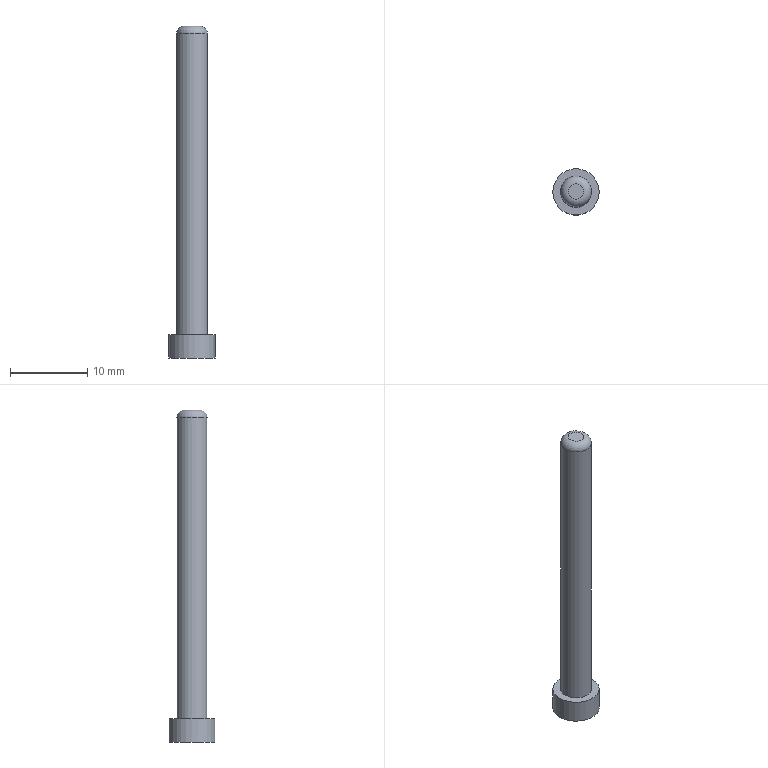Part | NX | features PG_666 2 | 1 solid | 6 faces | box 6 x 6 x 43 mm | volume 585.333 mm3 | plane 3 | cylinder 2 | torus 1 | commonest cylinder face diameters 4.001 x1 6 x1
STEP:
#1=CARTESIAN_POINT('',(3525.995,-894.948,862.716));
#2=VERTEX_POINT('',#1);
#3=CARTESIAN_POINT('',(3523.995,-894.948,862.716));
#4=DIRECTION('',(0.,0.,1.));
#5=DIRECTION('',(1.,0.,0.));
#6=AXIS2_PLACEMENT_3D('',#3,#4,#5);
#7=CIRCLE('',#6,2.001);
#8=EDGE_CURVE('',#2,#2,#7,.F.);
#9=ORIENTED_EDGE('',*,*,#8,.T.);
#10=EDGE_LOOP('',(#9));
#11=FACE_BOUND('',#10,.T.);
#12=CARTESIAN_POINT('',(3525.995,-894.948,823.716));
#13=VERTEX_POINT('',#12);
#14=CARTESIAN_POINT('',(3523.995,-894.948,823.716));
#15=DIRECTION('',(0.,0.,1.));
#16=DIRECTION('',(1.,0.,0.));
#17=AXIS2_PLACEMENT_3D('',#14,#15,#16);
#18=CIRCLE('',#17,2.001);
#19=EDGE_CURVE('',#13,#13,#18,.F.);
#20=ORIENTED_EDGE('',*,*,#19,.F.);
#21=EDGE_LOOP('',(#20));
#22=FACE_BOUND('',#21,.T.);
#23=CARTESIAN_POINT('',(3523.995,-894.948,858.716));
#24=DIRECTION('',(0.,0.,-1.));
#25=DIRECTION('',(-1.,0.,0.));
#26=AXIS2_PLACEMENT_3D('',#23,#24,#25);
#27=CYLINDRICAL_SURFACE('',#26,2.001);
#28=ADVANCED_FACE('',(#11,#22),#27,.T.);
#29=CARTESIAN_POINT('',(3524.995,-894.948,863.716));
#30=VERTEX_POINT('',#29);
#31=CARTESIAN_POINT('',(3523.995,-894.948,863.716));
#32=DIRECTION('',(0.,0.,1.));
#33=DIRECTION('',(1.,0.,0.));
#34=AXIS2_PLACEMENT_3D('',#31,#32,#33);
#35=CIRCLE('',#34,1.);
#36=EDGE_CURVE('',#30,#30,#35,.T.);
#37=ORIENTED_EDGE('',*,*,#36,.T.);
#38=EDGE_LOOP('',(#37));
#39=FACE_BOUND('',#38,.T.);
#40=CARTESIAN_POINT('',(3523.995,-894.948,863.716));
#41=DIRECTION('',(0.,0.,1.));
#42=DIRECTION('',(1.,0.,0.));
#43=AXIS2_PLACEMENT_3D('',#40,#41,#42);
#44=PLANE('',#43);
#45=ADVANCED_FACE('',(#39),#44,.T.);
#46=CARTESIAN_POINT('',(3520.995,-894.948,820.716));
#47=VERTEX_POINT('',#46);
#48=CARTESIAN_POINT('',(3523.995,-894.948,820.716));
#49=DIRECTION('',(0.,0.,1.));
#50=DIRECTION('',(-1.,0.,0.));
#51=AXIS2_PLACEMENT_3D('',#48,#49,#50);
#52=CIRCLE('',#51,3.);
#53=EDGE_CURVE('',#47,#47,#52,.T.);
#54=ORIENTED_EDGE('',*,*,#53,.F.);
#55=EDGE_LOOP('',(#54));
#56=FACE_BOUND('',#55,.T.);
#57=CARTESIAN_POINT('',(3523.995,-894.948,820.716));
#58=DIRECTION('',(0.,0.,-1.));
#59=DIRECTION('',(-1.,0.,0.));
#60=AXIS2_PLACEMENT_3D('',#57,#58,#59);
#61=PLANE('',#60);
#62=ADVANCED_FACE('',(#56),#61,.T.);
#63=ORIENTED_EDGE('',*,*,#19,.T.);
#64=EDGE_LOOP('',(#63));
#65=FACE_BOUND('',#64,.T.);
#66=CARTESIAN_POINT('',(3520.995,-894.948,823.716));
#67=VERTEX_POINT('',#66);
#68=CARTESIAN_POINT('',(3523.995,-894.948,823.716));
#69=DIRECTION('',(0.,0.,-1.));
#70=DIRECTION('',(-1.,0.,0.));
#71=AXIS2_PLACEMENT_3D('',#68,#69,#70);
#72=CIRCLE('',#71,3.);
#73=EDGE_CURVE('',#67,#67,#72,.T.);
#74=ORIENTED_EDGE('',*,*,#73,.F.);
#75=EDGE_LOOP('',(#74));
#76=FACE_BOUND('',#75,.T.);
#77=CARTESIAN_POINT('',(3523.995,-894.948,823.716));
#78=DIRECTION('',(0.,0.,1.));
#79=DIRECTION('',(1.,0.,0.));
#80=AXIS2_PLACEMENT_3D('',#77,#78,#79);
#81=PLANE('',#80);
#82=ADVANCED_FACE('',(#65,#76),#81,.T.);
#83=ORIENTED_EDGE('',*,*,#53,.T.);
#84=EDGE_LOOP('',(#83));
#85=FACE_BOUND('',#84,.T.);
#86=ORIENTED_EDGE('',*,*,#73,.T.);
#87=EDGE_LOOP('',(#86));
#88=FACE_BOUND('',#87,.T.);
#89=CARTESIAN_POINT('',(3523.995,-894.948,823.716));
#90=DIRECTION('',(0.,0.,-1.));
#91=DIRECTION('',(-1.,0.,0.));
#92=AXIS2_PLACEMENT_3D('',#89,#90,#91);
#93=CYLINDRICAL_SURFACE('',#92,3.);
#94=ADVANCED_FACE('',(#85,#88),#93,.T.);
#95=ORIENTED_EDGE('',*,*,#36,.F.);
#96=EDGE_LOOP('',(#95));
#97=FACE_BOUND('',#96,.T.);
#98=ORIENTED_EDGE('',*,*,#8,.F.);
#99=EDGE_LOOP('',(#98));
#100=FACE_BOUND('',#99,.T.);
#101=CARTESIAN_POINT('',(3523.995,-894.948,862.716));
#102=DIRECTION('',(0.,0.,1.));
#103=DIRECTION('',(1.,0.,0.));
#104=AXIS2_PLACEMENT_3D('',#101,#102,#103);
#105=TOROIDAL_SURFACE('',#104,1.,1.);
#106=ADVANCED_FACE('',(#97,#100),#105,.T.);
#107=CLOSED_SHELL('',(#28,#45,#62,#82,#94,#106));
#108=MANIFOLD_SOLID_BREP('',#107);
#109=(LENGTH_UNIT()NAMED_UNIT(*)SI_UNIT(.MILLI.,.METRE.));
#110=UNCERTAINTY_MEASURE_WITH_UNIT(LENGTH_MEASURE(0.00001),#109,'','');
#111=(NAMED_UNIT(*)PLANE_ANGLE_UNIT()SI_UNIT($,.RADIAN.));
#112=(NAMED_UNIT(*)SI_UNIT($,.STERADIAN.)SOLID_ANGLE_UNIT());
#113=(GEOMETRIC_REPRESENTATION_CONTEXT(3)GLOBAL_UNCERTAINTY_ASSIGNED_CONTEXT((#110))GLOBAL_UNIT_ASSIGNED_CONTEXT((#109,#111,#112))REPRESENTATION_CONTEXT('',''));
#114=ADVANCED_BREP_SHAPE_REPRESENTATION('',(#108),#113);